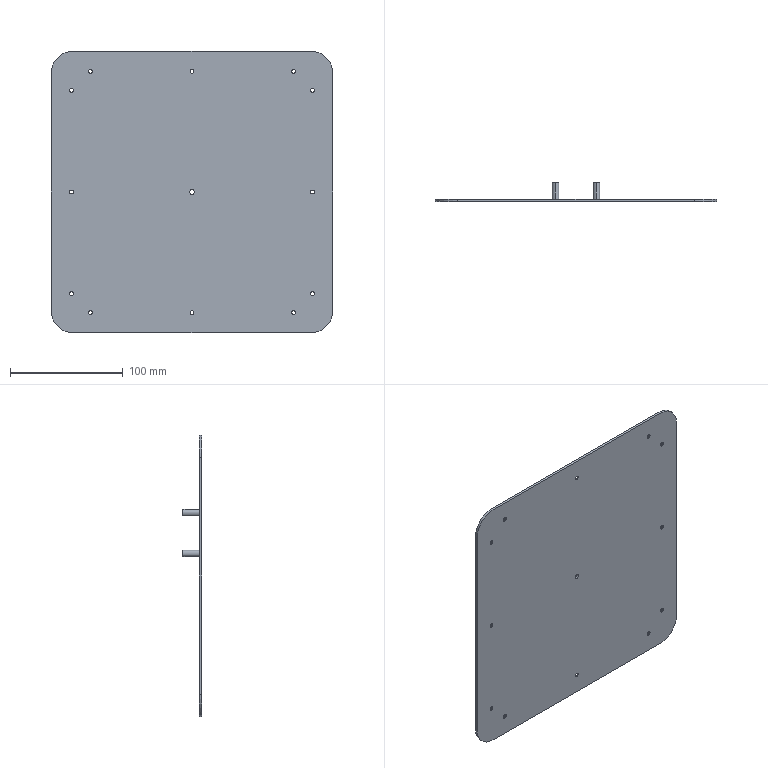Part | SolidWorks | features Chamfer 2, Extrusion 1, ICE 1 | 1 solid | 80 faces | box 249.5 x 17 x 249.5 mm | volume 125056 mm3 | cylinder 38 | cone 32 | plane 10 | commonest cylinder face diameters 3.5 x24 5.8 x8 40 x4 4 x2